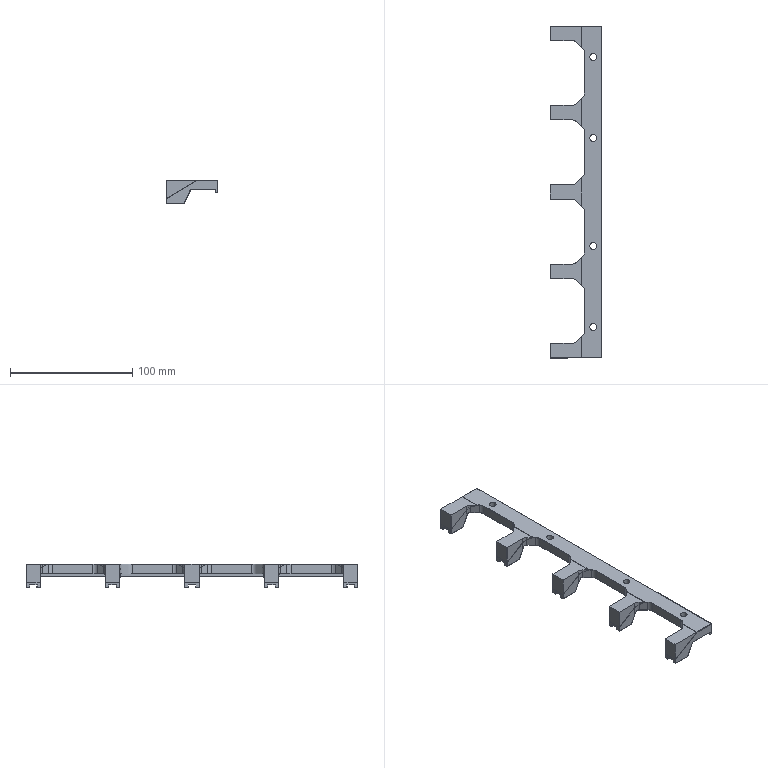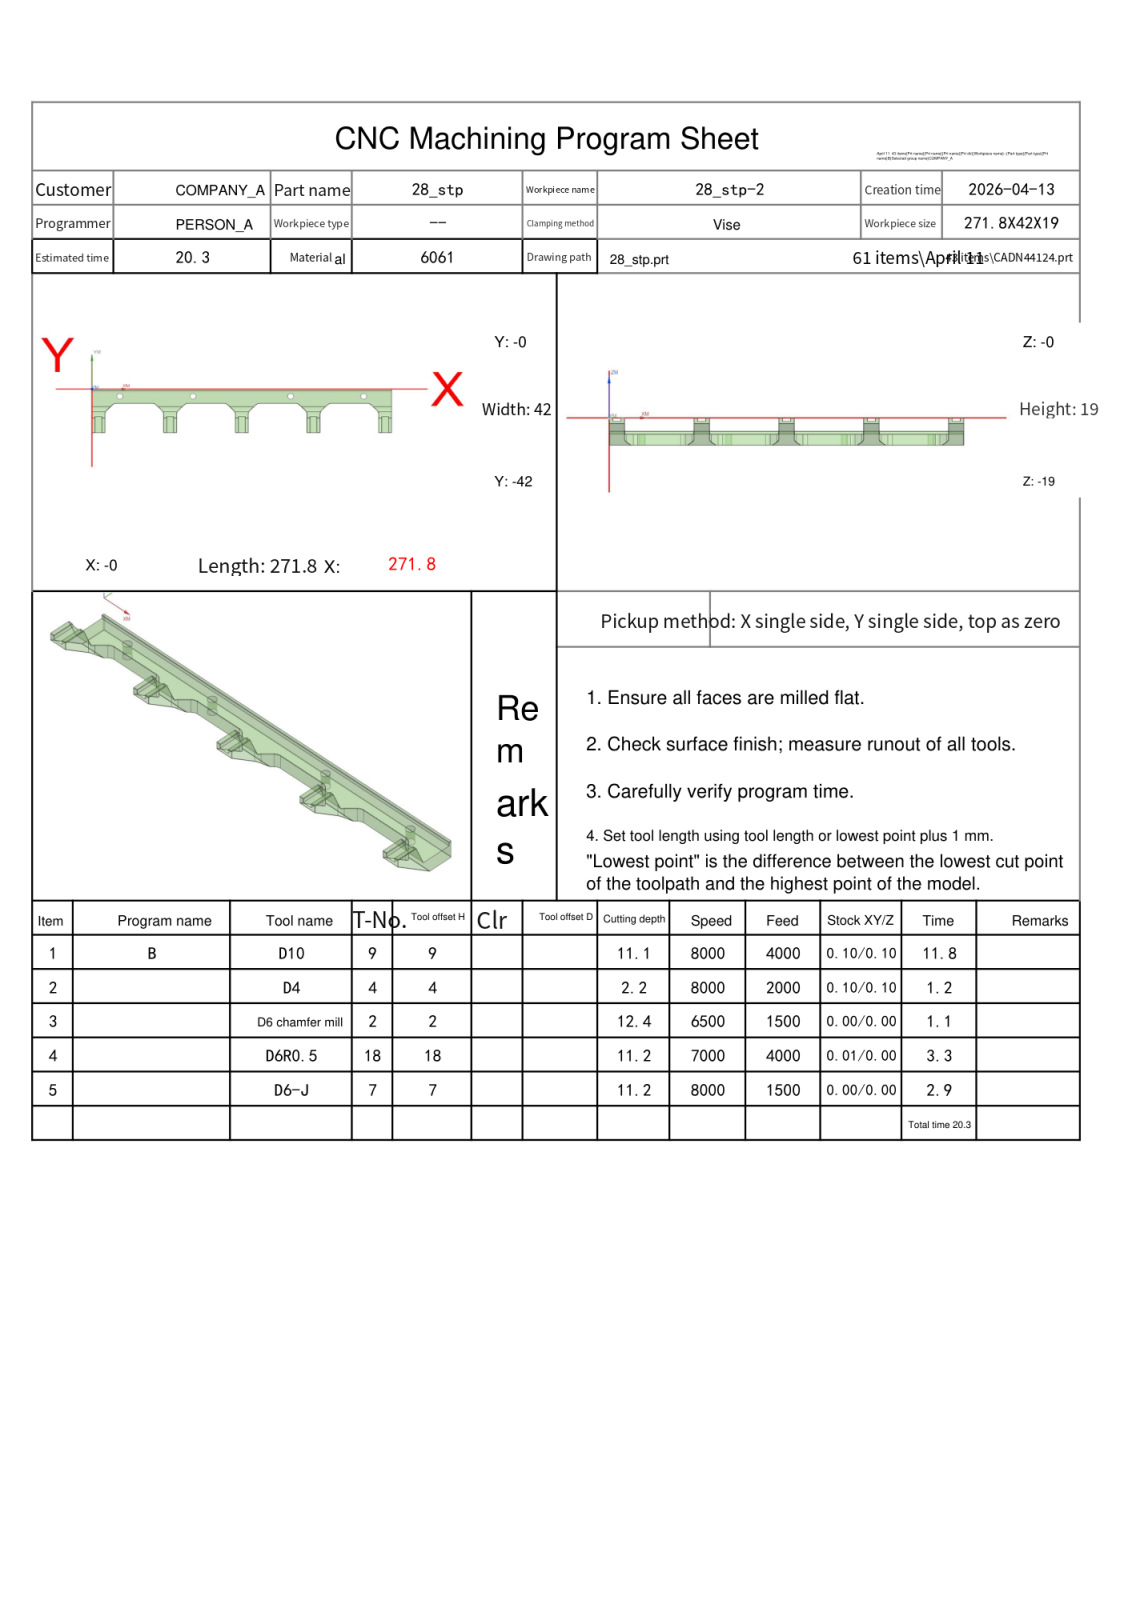NC program | NX | posted by the shop | part box 42 x 271.8 x 19 mm
Lines 13895 to 14465 of 14465:
N5 T07 M06
(D6-J  D=6. R=0. H=07 ce=0.40 di=0.00)
G00 G90 G54 X13.46 Y-23.649 M03 S7000
G43 H07 Z15.8
M08
Z1.5
G01 Z0.0 F1500.
G03 X12.5 Y-24.825 I.24 J-1.176
G01 Y-44.46
G02 X11.96 Y-45. I-.54 J0.0
G01 X10.575
G02 X9.975 Y-44.4 I0.0 J.6
G01 Y-25.425
G03 X9.375 Y-24.825 I-.6 J0.0
G01 X8.05
G03 X7.45 Y-25.425 I0.0 J-.6
G01 Y-44.4
G02 X6.85 Y-45. I-.6 J0.0
G01 X5.465
G02 X4.925 Y-44.46 I0.0 J.54
G01 Y-25.425
G03 X4.325 Y-24.825 I-.6 J0.0
G01 X4.223
X3.
G03 X2.4 Y-25.425 I0.0 J-.6
G01 Y-45.
G03 X3.6 Y-46.2 I1.2 J0.0
G01 Z1.5
G00 Z4.
X78.461 Y-23.649
Z1.5
G01 Z0.0
G03 X77.5 Y-24.825 I.238 J-1.176
G01 Y-44.46
G02 X76.96 Y-45. I-.54 J0.0
G01 X75.55
G02 X74.95 Y-44.4 I0.0 J.6
G01 Y-25.425
G03 X74.35 Y-24.825 I-.6 J0.0
G01 X73.
G03 X72.4 Y-25.425 I0.0 J-.6
G01 Y-44.4
G02 X71.8 Y-45. I-.6 J0.0
G01 X70.39
G02 X69.85 Y-44.46 I0.0 J.54
G01 Y-25.425
G03 X69.25 Y-24.825 I-.6 J0.0
G01 X69.219
X67.9
G03 X67.3 Y-25.425 I0.0 J-.6
G01 Y-45.
G03 X68.5 Y-46.2 I1.2 J0.0
G01 Z1.5
G00 Z4.
X143.457 Y-23.65
Z1.5
G01 Z0.0
G03 X142.5 Y-24.825 I.242 J-1.175
G01 Y-44.46
G02 X141.96 Y-45. I-.54 J0.0
G01 X140.55
G02 X139.95 Y-44.4 I0.0 J.6
G01 Y-25.425
G03 X139.35 Y-24.825 I-.6 J0.0
G01 X138.
G03 X137.4 Y-25.425 I0.0 J-.6
G01 Y-44.46
G02 X136.86 Y-45. I-.54 J0.0
G01 X135.45
G02 X134.85 Y-44.4 I0.0 J.6
G01 Y-25.425
G03 X134.25 Y-24.825 I-.6 J0.0
G01 X134.225
X132.9
G03 X132.3 Y-25.425 I0.0 J-.6
G01 Y-45.
G03 X133.5 Y-46.2 I1.2 J0.0
G01 Z1.5
G00 Z4.
X208.463 Y-23.649
Z1.5
G01 Z0.0
G03 X207.5 Y-24.825 I.237 J-1.176
G01 Y-44.46
G02 X206.96 Y-45. I-.54 J0.0
G01 X205.55
G02 X204.95 Y-44.4 I0.0 J.6
G01 Y-25.425
G03 X204.35 Y-24.825 I-.6 J0.0
G01 X203.
G03 X202.4 Y-25.425 I0.0 J-.6
G01 Y-44.46
G02 X201.86 Y-45. I-.54 J0.0
G01 X200.45
G02 X199.85 Y-44.4 I0.0 J.6
G01 Y-25.425
G03 X199.25 Y-24.825 I-.6 J0.0
G01 X199.221
X197.9
G03 X197.3 Y-25.425 I0.0 J-.6
G01 Y-45.
G03 X198.5 Y-46.2 I1.2 J0.0
G01 Z1.5
G00 Z4.
X273.36 Y-23.649
Z1.5
G01 Z0.0
G03 X272.4 Y-24.825 I.24 J-1.176
G01 Y-44.46
G02 X271.86 Y-45. I-.54 J0.0
G01 X270.475
G02 X269.875 Y-44.4 I0.0 J.6
G01 Y-25.425
G03 X269.275 Y-24.825 I-.6 J0.0
G01 X267.95
G03 X267.35 Y-25.425 I0.0 J-.6
G01 Y-44.4
G02 X266.75 Y-45. I-.6 J0.0
G01 X265.365
G02 X264.825 Y-44.46 I0.0 J.54
G01 Y-25.425
G03 X264.225 Y-24.825 I-.6 J0.0
G01 X264.217
X262.9
G03 X262.3 Y-25.425 I0.0 J-.6
G01 Y-45.
G03 X263.5 Y-46.2 I1.2 J0.0
G01 Z1.5
G00 Z15.8
G00 G90 X268.098 Y-46.391 M03 S8000
Z15.8
Z-1.3
G01 Z-2.3 F1000.
G41 D07
X268.156 Y-46.2
G03 X268.209 Y-45.849 I-1.147 J.351
X267.857 Y-45. I-1.2 J0.0
G01 X265.9 Y-43.043
Y-25.553
X267.758 Y-23.475
G03 X268.064 Y-22.675 I-.894 J.8
X267.995 Y-22.275 I-1.2 J0.0
G01 G40 X267.929 Y-22.086
X263.871
G41 D07
X263.805 Y-22.275
G03 X263.736 Y-22.675 I1.131 J-.4
X264.042 Y-23.475 I1.2 J0.0
G01 X265.9 Y-25.553
Y-43.043
X263.943 Y-45.
G03 X263.591 Y-45.849 I.849 J-.849
X263.644 Y-46.2 I1.2 J0.0
G01 G40 X263.702 Y-46.391
Z-1.3
G00 Z3.
X203.098
Z-1.3
G01 Z-2.3
G41 D07
X203.156 Y-46.2
G03 X203.209 Y-45.849 I-1.147 J.351
X202.857 Y-45. I-1.2 J0.0
G01 X200.9 Y-43.043
Y-25.553
X202.758 Y-23.475
G03 X203.064 Y-22.675 I-.894 J.8
X202.995 Y-22.275 I-1.2 J0.0
G01 G40 X202.929 Y-22.086
X198.871
G41 D07
X198.805 Y-22.275
G03 X198.736 Y-22.675 I1.131 J-.4
X199.042 Y-23.475 I1.2 J0.0
G01 X200.9 Y-25.553
Y-43.043
X198.943 Y-45.
G03 X198.591 Y-45.849 I.849 J-.849
X198.644 Y-46.2 I1.2 J0.0
G01 G40 X198.702 Y-46.391
Z-1.3
G00 Z3.
X138.098
Z-1.3
G01 Z-2.3
G41 D07
X138.156 Y-46.2
G03 X138.209 Y-45.849 I-1.147 J.351
X137.857 Y-45. I-1.2 J0.0
G01 X135.9 Y-43.043
Y-25.553
X137.758 Y-23.475
G03 X138.064 Y-22.675 I-.894 J.8
X137.995 Y-22.275 I-1.2 J0.0
G01 G40 X137.929 Y-22.086
X133.871
G41 D07
X133.805 Y-22.275
G03 X133.736 Y-22.675 I1.131 J-.4
X134.042 Y-23.475 I1.2 J0.0
G01 X135.9 Y-25.553
Y-43.043
X133.943 Y-45.
G03 X133.591 Y-45.849 I.849 J-.849
X133.644 Y-46.2 I1.2 J0.0
G01 G40 X133.702 Y-46.391
Z-1.3
G00 Z3.
X73.098
Z-1.3
G01 Z-2.3
G41 D07
X73.156 Y-46.2
G03 X73.209 Y-45.849 I-1.147 J.351
X72.857 Y-45. I-1.2 J0.0
G01 X70.9 Y-43.043
Y-25.553
X72.758 Y-23.475
G03 X73.064 Y-22.675 I-.894 J.8
X72.995 Y-22.275 I-1.2 J0.0
G01 G40 X72.929 Y-22.086
X68.871
G41 D07
X68.805 Y-22.275
G03 X68.736 Y-22.675 I1.131 J-.4
X69.042 Y-23.475 I1.2 J0.0
G01 X70.9 Y-25.553
Y-43.043
X68.943 Y-45.
G03 X68.591 Y-45.849 I.849 J-.849
X68.644 Y-46.2 I1.2 J0.0
G01 G40 X68.702 Y-46.391
Z-1.3
G00 Z3.
X8.098
Z-1.3
G01 Z-2.3
G41 D07
X8.156 Y-46.2
G03 X8.209 Y-45.849 I-1.147 J.351
X7.857 Y-45. I-1.2 J0.0
G01 X5.9 Y-43.043
Y-25.553
X7.758 Y-23.475
G03 X8.064 Y-22.675 I-.894 J.8
X7.995 Y-22.275 I-1.2 J0.0
G01 G40 X7.929 Y-22.086
X3.871
G41 D07
X3.805 Y-22.275
G03 X3.736 Y-22.675 I1.131 J-.4
X4.042 Y-23.475 I1.2 J0.0
G01 X5.9 Y-25.553
Y-43.043
X3.943 Y-45.
G03 X3.591 Y-45.849 I.849 J-.849
X3.644 Y-46.2 I1.2 J0.0
G01 G40 X3.702 Y-46.391
Z-1.3
G00 Z15.8
G00 G90 X137.1 Y-6.15 M03 S7000
Z15.8
Z-7.75
G01 Z-9.25 F1500.
Y-3.75
G03 X135.9 Y-2.55 I-1.2 J0.0
G01 X.097
G02 X-.322 Y-2.376 I.003 J.6
G01 X-.426 Y-2.272
G02 X-.6 Y-1.853 I.426 J.422
G01 Y-.497
G02 X-.426 Y-.078 I.6 J-.003
G01 X.078 Y.426
G02 X.497 Y.6 I.422 J-.426
G01 X271.303
G02 X271.724 Y.424 I-.003 J-.6
G01 X272.226 Y-.078
G02 X272.4 Y-.497 I-.426 J-.422
G01 Y-1.853
G02 X272.226 Y-2.272 I-.6 J.003
G01 X272.122 Y-2.376
G02 X271.703 Y-2.55 I-.422 J.426
G01 X135.9
X134.9
G03 X133.7 Y-3.75 I0.0 J-1.2
G01 Y-6.15
Z-7.75
G00 Z15.8
G00 G90 X151.509 Y-18.347 M03 S8000
Z15.8
Z-9.75
G01 Z-11.25 F1000.
X149.804 Y-16.642
G03 X148.955 Y-16.29 I-.849 J-.849
X148.107 Y-16.642 I0.0 J-1.2
G01 X145.122 Y-19.626
G02 X144.87 Y-19.73 I-.253 J.256
X144.561 Y-19.554 I0.0 J.36
G01 X144.001 Y-18.6
X127.799
X127.239 Y-19.554
G02 X126.93 Y-19.73 I-.309 J.184
X126.678 Y-19.626 I0.0 J.36
G01 X122.94 Y-15.889
G03 X119.829 Y-14.6 I-3.111 J-3.111
G01 X86.971
G03 X83.86 Y-15.889 I0.0 J-4.4
G01 X80.122 Y-19.626
G02 X79.87 Y-19.73 I-.253 J.256
X79.561 Y-19.554 I0.0 J.36
G01 X79.001 Y-18.6
X62.799
X62.239 Y-19.554
G02 X61.93 Y-19.73 I-.309 J.184
X61.678 Y-19.626 I0.0 J.36
G01 X57.94 Y-15.889
G03 X54.829 Y-14.6 I-3.111 J-3.111
G01 X21.971
G03 X18.86 Y-15.889 I0.0 J-4.4
G01 X15.122 Y-19.626
G02 X14.87 Y-19.73 I-.253 J.256
X14.561 Y-19.554 I0.0 J.36
G01 X14.001 Y-18.6
X-.004
G02 X-.6 Y-18.004 I.004 J.6
G01 Y-5.946
G02 X-.004 Y-5.35 I.6 J-.004
G01 X271.804
G02 X272.4 Y-5.946 I-.004 J-.6
G01 Y-18.004
G02 X271.804 Y-18.6 I-.6 J.003
G01 X258.579
X257.575 Y-19.723
G02 X257.175 Y-19.9 I-.4 J.362
X256.796 Y-19.744 I0.0 J.54
G01 X252.94 Y-15.889
G03 X249.829 Y-14.6 I-3.111 J-3.111
G01 X216.971
G03 X213.86 Y-15.889 I0.0 J-4.4
G01 X210.122 Y-19.626
G02 X209.87 Y-19.73 I-.253 J.256
X209.561 Y-19.554 I0.0 J.36
G01 X209.001 Y-18.6
X192.799
X192.239 Y-19.554
G02 X191.93 Y-19.73 I-.309 J.184
X191.678 Y-19.626 I0.0 J.36
G01 X187.94 Y-15.889
G03 X184.829 Y-14.6 I-3.111 J-3.111
G01 X151.971
G03 X148.86 Y-15.889 I0.0 J-4.4
G01 X145.985 Y-18.763
G02 X145.561 Y-18.939 I-.424 J.424
X145.039 Y-18.634 I0.0 J.6
G01 X143.495 Y-15.904
G03 X142.973 Y-15.6 I-.522 J-.296
G01 X127.799
G03 X127.291 Y-15.643 I0.0 J-3.
G01 X127.194 Y-15.651
G02 X126.773 Y-15.479 I0.0 J.6
G01 X125.062 Y-13.767
G03 X119.829 Y-11.6 I-5.233 J-5.233
G01 X86.971
G03 X81.738 Y-13.767 I0.0 J-7.4
G01 X80.027 Y-15.479
G02 X79.606 Y-15.651 I-.421 J.427
G01 X79.509 Y-15.643
G03 X79.001 Y-15.6 I-.509 J-2.957
G01 X62.799
G03 X62.291 Y-15.643 I0.0 J-3.
G01 X62.194 Y-15.651
G02 X61.773 Y-15.479 I0.0 J.6
G01 X60.062 Y-13.767
G03 X54.829 Y-11.6 I-5.233 J-5.233
G01 X21.971
G03 X16.738 Y-13.767 I0.0 J-7.4
G01 X15.027 Y-15.479
G02 X14.606 Y-15.651 I-.421 J.427
G01 X14.509 Y-15.643
G03 X14.001 Y-15.6 I-.508 J-2.957
G01 X2.996
G02 X2.4 Y-15.004 I.004 J.6
G01 Y-8.946
G02 X2.996 Y-8.35 I.6 J-.004
G01 X11.599
G02 X12.135 Y-8.682 I0.0 J-.6
G01 X13.34 Y-11.091
G03 X13.671 Y-11.386 I.537 J.269
G02 X14.065 Y-11.95 I-.206 J-.564
X13.892 Y-12.371 I-.6 J0.0
G01 X13.836 Y-12.428
G02 X13.419 Y-12.6 I-.421 J.428
G01 X5.995
G02 X5.4 Y-12.005 I.005 J.6
G01 Y-11.945
G02 X5.995 Y-11.35 I.6 J-.005
G01 X11.721
G03 X12.145 Y-11.174 I0.0 J.6
G01 X14.794 Y-8.525
G02 X15.217 Y-8.35 I.424 J-.425
G01 X76.599
G02 X77.135 Y-8.682 I0.0 J-.6
G01 X78.34 Y-11.091
G03 X78.671 Y-11.386 I.537 J.269
G02 X79.065 Y-11.95 I-.206 J-.564
X78.892 Y-12.371 I-.6 J0.0
G01 X78.836 Y-12.428
G02 X78.419 Y-12.6 I-.421 J.428
G01 X63.381
G02 X62.964 Y-12.428 I.005 J.6
G01 X62.908 Y-12.371
G02 X62.735 Y-11.95 I.428 J.421
X63.331 Y-11.35 I.6 J0.0
G01 X76.721
G03 X77.145 Y-11.174 I0.0 J.6
G01 X79.794 Y-8.525
G02 X80.217 Y-8.35 I.424 J-.425
G01 X268.804
G02 X269.4 Y-8.946 I-.004 J-.6
G01 Y-15.004
G02 X268.804 Y-15.6 I-.6 J.004
G01 X258.579
G03 X257.557 Y-15.78 I0.0 J-3.
G02 X257.357 Y-15.814 I-.2 J.566
G01 X257.31 Y-15.812
G02 X256.923 Y-15.394 I.032 J.419
G01 X256.944 Y-15.261
X257.816 Y-12.645
X257.847 Y-12.456
G03 X257.791 Y-12.203 I-.6 J0.0
G02 X257.735 Y-11.95 I.544 J.253
X258.331 Y-11.35 I.6 J0.0
G01 X265.805
G02 X266.4 Y-11.945 I-.005 J-.6
G01 Y-12.005
G02 X265.805 Y-12.6 I-.6 J.005
G01 X259.391
X259.284 Y-12.61
X254.994 Y-13.392
X254.886 Y-13.402
G02 X254.507 Y-13.267 I0.0 J.6
G03 X249.829 Y-11.6 I-4.678 J-5.733
G01 X216.971
G03 X211.738 Y-13.767 I0.0 J-7.4
G01 X210.027 Y-15.479
G02 X209.606 Y-15.651 I-.421 J.427
G01 X209.509 Y-15.643
G03 X209.001 Y-15.6 I-.508 J-2.957
G01 X192.799
G03 X192.374 Y-15.63 I0.0 J-3.
G01 X192.323 Y-15.634
G02 X191.963 Y-15.274 I0.0 J.36
G01 X191.981 Y-15.161
X192.817 Y-12.645
X192.847 Y-12.456
G03 X192.791 Y-12.203 I-.6 J0.0
G02 X192.735 Y-11.95 I.544 J.253
X193.331 Y-11.35 I.6 J0.0
G01 X208.469
G02 X209.065 Y-11.95 I-.005 J-.6
X208.892 Y-12.371 I-.6 J0.0
G01 X208.836 Y-12.428
G02 X208.419 Y-12.6 I-.421 J.428
G01 X194.393
X194.286 Y-12.61
X189.994 Y-13.392
X189.886 Y-13.402
G02 X189.507 Y-13.267 I0.0 J.6
G03 X184.829 Y-11.6 I-4.678 J-5.733
G01 X151.971
G03 X146.738 Y-13.767 I0.0 J-7.4
G01 X146.222 Y-14.284
G02 X145.798 Y-14.46 I-.424 J.424
X145.517 Y-14.39 I0.0 J.6
G01 X142.268 Y-12.67
G03 X141.988 Y-12.6 I-.281 J-.53
G01 X128.381
G02 X127.964 Y-12.428 I.005 J.6
G01 X127.908 Y-12.371
G02 X127.735 Y-11.95 I.428 J.421
X128.331 Y-11.35 I.6 J0.0
G01 X143.469
G02 X144.065 Y-11.95 I-.005 J-.6
X143.892 Y-12.371 I-.6 J0.0
G01 X143.836 Y-12.428
G02 X143.632 Y-12.559 I-.421 J.428
X143.419 Y-12.6 I-.217 J.559
G01 X142.637
G03 X141.437 Y-13.8 I0.0 J-1.2
G01 Z-9.75
G00 Z15.8
G00 G90 X125.131 Y-22.988 M03 S8000
Z15.8
Z-10.25
G01 Z-11.25 F1000.
G41 D07
X125.324 Y-22.935
G03 X126.043 Y-22.385 I-.317 J1.157
G01 X128.028 Y-19.
X143.771
X145.758 Y-22.385
G03 X146.476 Y-22.935 I1.035 J.607
G01 G40 X146.669 Y-22.988
Z-10.25
G00 X190.131
G01 Z-11.25
G41 D07
X190.324 Y-22.935
G03 X191.043 Y-22.385 I-.317 J1.157
G01 X193.028 Y-19.
X208.772
X210.757 Y-22.385
G03 X211.476 Y-22.935 I1.035 J.607
G01 G40 X211.669 Y-22.988
Z-10.25
G00 X255.5 Y-25.161
G01 Z-11.25
G41 D07
X255.7
G03 X256.9 Y-23.961 I0.0 J1.2
G01 Y-21.078
X258.758 Y-19.
X272.942
X274.797 Y-21.074
G03 X275.691 Y-21.474 I.894 J.8
X276. Y-21.434 I0.0 J1.2
G01 G40 X276.193 Y-21.383
Z-10.25
G00 X276.191 Y-2.852
G01 Z-11.25
G41 D07
X276. Y-2.794
G03 X275.649 Y-2.741 I-.351 J-1.147
X274.8 Y-3.093 I0.0 J-1.2
G01 X272.943 Y-4.95
X-1.143
X-3. Y-3.093
G03 X-3.849 Y-2.741 I-.849 J-.849
X-4.2 Y-2.794 I0.0 J-1.2
G01 G40 X-4.391 Y-2.852
Z-10.25
G00 X-4.393 Y-21.383
G01 Z-11.25
G41 D07
X-4.2 Y-21.434
G03 X-3.891 Y-21.474 I.309 J1.16
X-2.997 Y-21.074 I0.0 J1.2
G01 X-1.142 Y-19.
X13.771
X15.758 Y-22.385
G03 X16.476 Y-22.935 I1.035 J.607
G01 G40 X16.669 Y-22.988
Z-10.25
G00 X60.131
G01 Z-11.25
G41 D07
X60.324 Y-22.935
G03 X61.043 Y-22.385 I-.317 J1.157
G01 X63.028 Y-19.
X78.771
X80.758 Y-22.385
G03 X81.476 Y-22.935 I1.035 J.607
G01 G40 X81.669 Y-22.988
Z-10.25
G00 Z15.8
M05
M09
G91 G28 Z0.0
G91 G28 Y0.0
M30
%